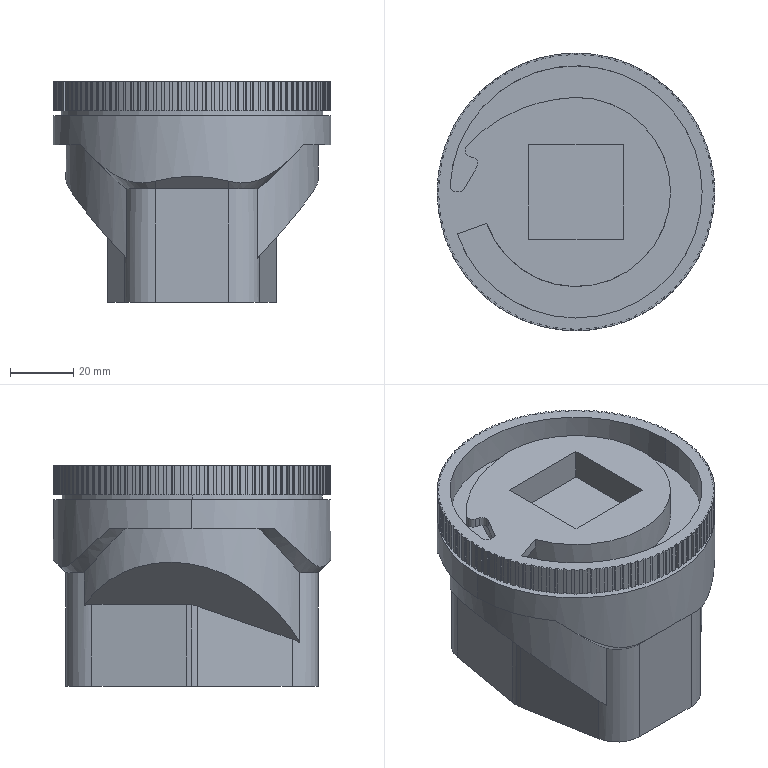Part | SolidWorks | features ICE 7, Chamfer 3, Fillet 2, CirPattern 1, Extrusion 1, RevCut 1 | 1 solid | 483 faces | box 88 x 88 x 70 mm | volume 300760 mm3 | plane 347 | cylinder 129 | cone 6 | spline 1 | commonest cylinder face diameters 88 x108 20 x8 80 x5 4 x4 60 x2 83 x2